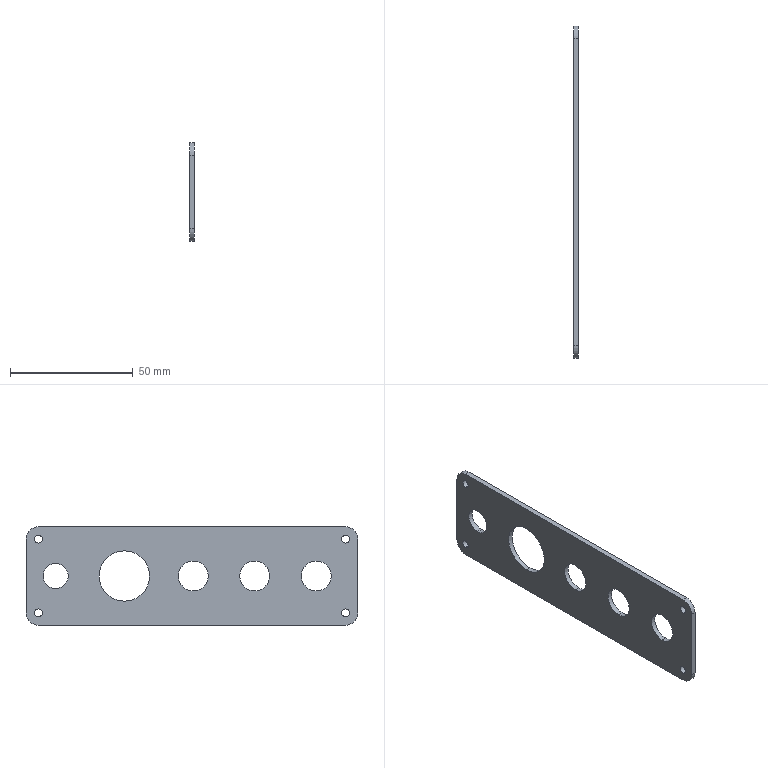Part | SolidWorks | features BaseBody 1 | 1 solid | 28 faces | box 2 x 135 x 40 mm | volume 9168 mm3 | cylinder 22 | plane 6 | commonest cylinder face diameters 3.2 x8 12.2 x6 10 x4 10.2 x2 20.5 x2
STEP:
#1=CARTESIAN_POINT('',(330.1,5.5,36.9));
#2=VERTEX_POINT('',#1);
#3=CARTESIAN_POINT('',(330.1,5.5,40.1));
#4=VERTEX_POINT('',#3);
#5=CARTESIAN_POINT('',(330.1,5.5,38.5));
#6=DIRECTION('',(-1.,0.,0.));
#7=DIRECTION('',(0.,0.,1.));
#8=AXIS2_PLACEMENT_3D('',#5,#6,#7);
#9=CIRCLE('',#8,1.6);
#10=EDGE_CURVE('',#2,#4,#9,.T.);
#11=ORIENTED_EDGE('',*,*,#10,.F.);
#12=CARTESIAN_POINT('',(328.1,5.5,36.9));
#13=VERTEX_POINT('',#12);
#14=CARTESIAN_POINT('',(330.1,5.5,36.9));
#15=DIRECTION('',(-1.,0.,0.));
#16=VECTOR('',#15,1000.);
#17=LINE('',#14,#16);
#18=EDGE_CURVE('',#2,#13,#17,.T.);
#19=ORIENTED_EDGE('',*,*,#18,.T.);
#20=CARTESIAN_POINT('',(328.1,5.5,40.1));
#21=VERTEX_POINT('',#20);
#22=CARTESIAN_POINT('',(328.1,5.5,38.5));
#23=DIRECTION('',(1.,0.,0.));
#24=DIRECTION('',(0.,0.,1.));
#25=AXIS2_PLACEMENT_3D('',#22,#23,#24);
#26=CIRCLE('',#25,1.6);
#27=EDGE_CURVE('',#21,#13,#26,.T.);
#28=ORIENTED_EDGE('',*,*,#27,.F.);
#29=CARTESIAN_POINT('',(330.1,5.5,40.1));
#30=DIRECTION('',(-1.,0.,0.));
#31=VECTOR('',#30,1000.);
#32=LINE('',#29,#31);
#33=EDGE_CURVE('',#4,#21,#32,.T.);
#34=ORIENTED_EDGE('',*,*,#33,.F.);
#35=EDGE_LOOP('',(#11,#19,#28,#34));
#36=FACE_OUTER_BOUND('',#35,.T.);
#37=CARTESIAN_POINT('',(330.1,5.5,38.5));
#38=DIRECTION('',(-1.,0.,0.));
#39=DIRECTION('',(0.,0.,1.));
#40=AXIS2_PLACEMENT_3D('',#37,#38,#39);
#41=CYLINDRICAL_SURFACE('',#40,1.6);
#42=ADVANCED_FACE('',(#36),#41,.F.);
#43=CARTESIAN_POINT('',(330.1,130.5,6.9));
#44=VERTEX_POINT('',#43);
#45=CARTESIAN_POINT('',(330.1,130.5,10.1));
#46=VERTEX_POINT('',#45);
#47=CARTESIAN_POINT('',(330.1,130.5,8.5));
#48=DIRECTION('',(-1.,0.,0.));
#49=DIRECTION('',(0.,0.,1.));
#50=AXIS2_PLACEMENT_3D('',#47,#48,#49);
#51=CIRCLE('',#50,1.6);
#52=EDGE_CURVE('',#44,#46,#51,.T.);
#53=ORIENTED_EDGE('',*,*,#52,.F.);
#54=CARTESIAN_POINT('',(328.1,130.5,6.9));
#55=VERTEX_POINT('',#54);
#56=CARTESIAN_POINT('',(330.1,130.5,6.9));
#57=DIRECTION('',(-1.,0.,0.));
#58=VECTOR('',#57,1000.);
#59=LINE('',#56,#58);
#60=EDGE_CURVE('',#44,#55,#59,.T.);
#61=ORIENTED_EDGE('',*,*,#60,.T.);
#62=CARTESIAN_POINT('',(328.1,130.5,10.1));
#63=VERTEX_POINT('',#62);
#64=CARTESIAN_POINT('',(328.1,130.5,8.5));
#65=DIRECTION('',(1.,0.,0.));
#66=DIRECTION('',(0.,0.,1.));
#67=AXIS2_PLACEMENT_3D('',#64,#65,#66);
#68=CIRCLE('',#67,1.6);
#69=EDGE_CURVE('',#63,#55,#68,.T.);
#70=ORIENTED_EDGE('',*,*,#69,.F.);
#71=CARTESIAN_POINT('',(330.1,130.5,10.1));
#72=DIRECTION('',(-1.,0.,0.));
#73=VECTOR('',#72,1000.);
#74=LINE('',#71,#73);
#75=EDGE_CURVE('',#46,#63,#74,.T.);
#76=ORIENTED_EDGE('',*,*,#75,.F.);
#77=EDGE_LOOP('',(#53,#61,#70,#76));
#78=FACE_OUTER_BOUND('',#77,.T.);
#79=CARTESIAN_POINT('',(330.1,130.5,8.5));
#80=DIRECTION('',(-1.,0.,0.));
#81=DIRECTION('',(0.,0.,1.));
#82=AXIS2_PLACEMENT_3D('',#79,#80,#81);
#83=CYLINDRICAL_SURFACE('',#82,1.6);
#84=ADVANCED_FACE('',(#78),#83,.F.);
#85=CARTESIAN_POINT('',(330.1,130.5,36.9));
#86=VERTEX_POINT('',#85);
#87=CARTESIAN_POINT('',(330.1,130.5,40.1));
#88=VERTEX_POINT('',#87);
#89=CARTESIAN_POINT('',(330.1,130.5,38.5));
#90=DIRECTION('',(-1.,0.,0.));
#91=DIRECTION('',(0.,0.,1.));
#92=AXIS2_PLACEMENT_3D('',#89,#90,#91);
#93=CIRCLE('',#92,1.6);
#94=EDGE_CURVE('',#86,#88,#93,.T.);
#95=ORIENTED_EDGE('',*,*,#94,.F.);
#96=CARTESIAN_POINT('',(328.1,130.5,36.9));
#97=VERTEX_POINT('',#96);
#98=CARTESIAN_POINT('',(330.1,130.5,36.9));
#99=DIRECTION('',(-1.,0.,0.));
#100=VECTOR('',#99,1000.);
#101=LINE('',#98,#100);
#102=EDGE_CURVE('',#86,#97,#101,.T.);
#103=ORIENTED_EDGE('',*,*,#102,.T.);
#104=CARTESIAN_POINT('',(328.1,130.5,40.1));
#105=VERTEX_POINT('',#104);
#106=CARTESIAN_POINT('',(328.1,130.5,38.5));
#107=DIRECTION('',(1.,0.,0.));
#108=DIRECTION('',(0.,0.,1.));
#109=AXIS2_PLACEMENT_3D('',#106,#107,#108);
#110=CIRCLE('',#109,1.6);
#111=EDGE_CURVE('',#105,#97,#110,.T.);
#112=ORIENTED_EDGE('',*,*,#111,.F.);
#113=CARTESIAN_POINT('',(330.1,130.5,40.1));
#114=DIRECTION('',(-1.,0.,0.));
#115=VECTOR('',#114,1000.);
#116=LINE('',#113,#115);
#117=EDGE_CURVE('',#88,#105,#116,.T.);
#118=ORIENTED_EDGE('',*,*,#117,.F.);
#119=EDGE_LOOP('',(#95,#103,#112,#118));
#120=FACE_OUTER_BOUND('',#119,.T.);
#121=CARTESIAN_POINT('',(330.1,130.5,38.5));
#122=DIRECTION('',(-1.,0.,0.));
#123=DIRECTION('',(0.,0.,1.));
#124=AXIS2_PLACEMENT_3D('',#121,#122,#123);
#125=CYLINDRICAL_SURFACE('',#124,1.6);
#126=ADVANCED_FACE('',(#120),#125,.F.);
#127=CARTESIAN_POINT('',(330.1,5.5,6.9));
#128=VERTEX_POINT('',#127);
#129=CARTESIAN_POINT('',(330.1,5.5,10.1));
#130=VERTEX_POINT('',#129);
#131=CARTESIAN_POINT('',(330.1,5.5,8.5));
#132=DIRECTION('',(-1.,0.,0.));
#133=DIRECTION('',(0.,0.,1.));
#134=AXIS2_PLACEMENT_3D('',#131,#132,#133);
#135=CIRCLE('',#134,1.6);
#136=EDGE_CURVE('',#128,#130,#135,.T.);
#137=ORIENTED_EDGE('',*,*,#136,.F.);
#138=CARTESIAN_POINT('',(328.1,5.5,6.9));
#139=VERTEX_POINT('',#138);
#140=CARTESIAN_POINT('',(330.1,5.5,6.9));
#141=DIRECTION('',(-1.,0.,0.));
#142=VECTOR('',#141,1000.);
#143=LINE('',#140,#142);
#144=EDGE_CURVE('',#128,#139,#143,.T.);
#145=ORIENTED_EDGE('',*,*,#144,.T.);
#146=CARTESIAN_POINT('',(328.1,5.5,10.1));
#147=VERTEX_POINT('',#146);
#148=CARTESIAN_POINT('',(328.1,5.5,8.5));
#149=DIRECTION('',(1.,0.,0.));
#150=DIRECTION('',(0.,0.,1.));
#151=AXIS2_PLACEMENT_3D('',#148,#149,#150);
#152=CIRCLE('',#151,1.6);
#153=EDGE_CURVE('',#147,#139,#152,.T.);
#154=ORIENTED_EDGE('',*,*,#153,.F.);
#155=CARTESIAN_POINT('',(330.1,5.5,10.1));
#156=DIRECTION('',(-1.,0.,0.));
#157=VECTOR('',#156,1000.);
#158=LINE('',#155,#157);
#159=EDGE_CURVE('',#130,#147,#158,.T.);
#160=ORIENTED_EDGE('',*,*,#159,.F.);
#161=EDGE_LOOP('',(#137,#145,#154,#160));
#162=FACE_OUTER_BOUND('',#161,.T.);
#163=CARTESIAN_POINT('',(330.1,5.5,8.5));
#164=DIRECTION('',(-1.,0.,0.));
#165=DIRECTION('',(0.,0.,1.));
#166=AXIS2_PLACEMENT_3D('',#163,#164,#165);
#167=CYLINDRICAL_SURFACE('',#166,1.6);
#168=ADVANCED_FACE('',(#162),#167,.F.);
#169=CARTESIAN_POINT('',(330.1,95.5,13.25));
#170=VERTEX_POINT('',#169);
#171=CARTESIAN_POINT('',(330.1,95.5,33.75));
#172=VERTEX_POINT('',#171);
#173=CARTESIAN_POINT('',(330.1,95.5,23.5));
#174=DIRECTION('',(-1.,0.,0.));
#175=DIRECTION('',(0.,0.,1.));
#176=AXIS2_PLACEMENT_3D('',#173,#174,#175);
#177=CIRCLE('',#176,10.25);
#178=EDGE_CURVE('',#170,#172,#177,.T.);
#179=ORIENTED_EDGE('',*,*,#178,.F.);
#180=CARTESIAN_POINT('',(328.1,95.5,13.25));
#181=VERTEX_POINT('',#180);
#182=CARTESIAN_POINT('',(342.1,95.5,13.25));
#183=DIRECTION('',(-1.,0.,0.));
#184=VECTOR('',#183,1000.);
#185=LINE('',#182,#184);
#186=EDGE_CURVE('',#170,#181,#185,.T.);
#187=ORIENTED_EDGE('',*,*,#186,.T.);
#188=CARTESIAN_POINT('',(328.1,95.5,33.75));
#189=VERTEX_POINT('',#188);
#190=CARTESIAN_POINT('',(328.1,95.5,23.5));
#191=DIRECTION('',(1.,0.,0.));
#192=DIRECTION('',(0.,0.,1.));
#193=AXIS2_PLACEMENT_3D('',#190,#191,#192);
#194=CIRCLE('',#193,10.25);
#195=EDGE_CURVE('',#189,#181,#194,.T.);
#196=ORIENTED_EDGE('',*,*,#195,.F.);
#197=CARTESIAN_POINT('',(342.1,95.5,33.75));
#198=DIRECTION('',(-1.,0.,0.));
#199=VECTOR('',#198,1000.);
#200=LINE('',#197,#199);
#201=EDGE_CURVE('',#172,#189,#200,.T.);
#202=ORIENTED_EDGE('',*,*,#201,.F.);
#203=EDGE_LOOP('',(#179,#187,#196,#202));
#204=FACE_OUTER_BOUND('',#203,.T.);
#205=CARTESIAN_POINT('',(342.1,95.5,23.5));
#206=DIRECTION('',(-1.,0.,0.));
#207=DIRECTION('',(0.,0.,1.));
#208=AXIS2_PLACEMENT_3D('',#205,#206,#207);
#209=CYLINDRICAL_SURFACE('',#208,10.25);
#210=ADVANCED_FACE('',(#204),#209,.F.);
#211=CARTESIAN_POINT('',(330.1,123.5,18.4));
#212=VERTEX_POINT('',#211);
#213=CARTESIAN_POINT('',(330.1,123.5,28.6));
#214=VERTEX_POINT('',#213);
#215=CARTESIAN_POINT('',(330.1,123.5,23.5));
#216=DIRECTION('',(-1.,0.,0.));
#217=DIRECTION('',(0.,0.,1.));
#218=AXIS2_PLACEMENT_3D('',#215,#216,#217);
#219=CIRCLE('',#218,5.1);
#220=EDGE_CURVE('',#212,#214,#219,.T.);
#221=ORIENTED_EDGE('',*,*,#220,.F.);
#222=CARTESIAN_POINT('',(328.1,123.5,18.4));
#223=VERTEX_POINT('',#222);
#224=CARTESIAN_POINT('',(330.1,123.5,18.4));
#225=DIRECTION('',(-1.,0.,0.));
#226=VECTOR('',#225,1000.);
#227=LINE('',#224,#226);
#228=EDGE_CURVE('',#212,#223,#227,.T.);
#229=ORIENTED_EDGE('',*,*,#228,.T.);
#230=CARTESIAN_POINT('',(328.1,123.5,28.6));
#231=VERTEX_POINT('',#230);
#232=CARTESIAN_POINT('',(328.1,123.5,23.5));
#233=DIRECTION('',(1.,0.,0.));
#234=DIRECTION('',(0.,0.,1.));
#235=AXIS2_PLACEMENT_3D('',#232,#233,#234);
#236=CIRCLE('',#235,5.1);
#237=EDGE_CURVE('',#231,#223,#236,.T.);
#238=ORIENTED_EDGE('',*,*,#237,.F.);
#239=CARTESIAN_POINT('',(330.1,123.5,28.6));
#240=DIRECTION('',(-1.,0.,0.));
#241=VECTOR('',#240,1000.);
#242=LINE('',#239,#241);
#243=EDGE_CURVE('',#214,#231,#242,.T.);
#244=ORIENTED_EDGE('',*,*,#243,.F.);
#245=EDGE_LOOP('',(#221,#229,#238,#244));
#246=FACE_OUTER_BOUND('',#245,.T.);
#247=CARTESIAN_POINT('',(330.1,123.5,23.5));
#248=DIRECTION('',(-1.,0.,0.));
#249=DIRECTION('',(0.,0.,1.));
#250=AXIS2_PLACEMENT_3D('',#247,#248,#249);
#251=CYLINDRICAL_SURFACE('',#250,5.1);
#252=ADVANCED_FACE('',(#246),#251,.F.);
#253=CARTESIAN_POINT('',(330.1,67.5,17.4));
#254=VERTEX_POINT('',#253);
#255=CARTESIAN_POINT('',(330.1,67.5,29.6));
#256=VERTEX_POINT('',#255);
#257=CARTESIAN_POINT('',(330.1,67.5,23.5));
#258=DIRECTION('',(-1.,0.,0.));
#259=DIRECTION('',(0.,0.,1.));
#260=AXIS2_PLACEMENT_3D('',#257,#258,#259);
#261=CIRCLE('',#260,6.1);
#262=EDGE_CURVE('',#254,#256,#261,.T.);
#263=ORIENTED_EDGE('',*,*,#262,.F.);
#264=CARTESIAN_POINT('',(328.1,67.5,17.4));
#265=VERTEX_POINT('',#264);
#266=CARTESIAN_POINT('',(342.1,67.5,17.4));
#267=DIRECTION('',(-1.,0.,0.));
#268=VECTOR('',#267,1000.);
#269=LINE('',#266,#268);
#270=EDGE_CURVE('',#254,#265,#269,.T.);
#271=ORIENTED_EDGE('',*,*,#270,.T.);
#272=CARTESIAN_POINT('',(328.1,67.5,29.6));
#273=VERTEX_POINT('',#272);
#274=CARTESIAN_POINT('',(328.1,67.5,23.5));
#275=DIRECTION('',(1.,0.,0.));
#276=DIRECTION('',(0.,0.,1.));
#277=AXIS2_PLACEMENT_3D('',#274,#275,#276);
#278=CIRCLE('',#277,6.1);
#279=EDGE_CURVE('',#273,#265,#278,.T.);
#280=ORIENTED_EDGE('',*,*,#279,.F.);
#281=CARTESIAN_POINT('',(342.1,67.5,29.6));
#282=DIRECTION('',(-1.,0.,0.));
#283=VECTOR('',#282,1000.);
#284=LINE('',#281,#283);
#285=EDGE_CURVE('',#256,#273,#284,.T.);
#286=ORIENTED_EDGE('',*,*,#285,.F.);
#287=EDGE_LOOP('',(#263,#271,#280,#286));
#288=FACE_OUTER_BOUND('',#287,.T.);
#289=CARTESIAN_POINT('',(342.1,67.5,23.5));
#290=DIRECTION('',(-1.,0.,0.));
#291=DIRECTION('',(0.,0.,1.));
#292=AXIS2_PLACEMENT_3D('',#289,#290,#291);
#293=CYLINDRICAL_SURFACE('',#292,6.1);
#294=ADVANCED_FACE('',(#288),#293,.F.);
#295=CARTESIAN_POINT('',(330.1,42.5,17.4));
#296=VERTEX_POINT('',#295);
#297=CARTESIAN_POINT('',(330.1,42.5,29.6));
#298=VERTEX_POINT('',#297);
#299=CARTESIAN_POINT('',(330.1,42.5,23.5));
#300=DIRECTION('',(-1.,0.,0.));
#301=DIRECTION('',(0.,0.,1.));
#302=AXIS2_PLACEMENT_3D('',#299,#300,#301);
#303=CIRCLE('',#302,6.1);
#304=EDGE_CURVE('',#296,#298,#303,.T.);
#305=ORIENTED_EDGE('',*,*,#304,.F.);
#306=CARTESIAN_POINT('',(328.1,42.5,17.4));
#307=VERTEX_POINT('',#306);
#308=CARTESIAN_POINT('',(342.1,42.5,17.4));
#309=DIRECTION('',(-1.,0.,0.));
#310=VECTOR('',#309,1000.);
#311=LINE('',#308,#310);
#312=EDGE_CURVE('',#296,#307,#311,.T.);
#313=ORIENTED_EDGE('',*,*,#312,.T.);
#314=CARTESIAN_POINT('',(328.1,42.5,29.6));
#315=VERTEX_POINT('',#314);
#316=CARTESIAN_POINT('',(328.1,42.5,23.5));
#317=DIRECTION('',(1.,0.,0.));
#318=DIRECTION('',(0.,0.,1.));
#319=AXIS2_PLACEMENT_3D('',#316,#317,#318);
#320=CIRCLE('',#319,6.1);
#321=EDGE_CURVE('',#315,#307,#320,.T.);
#322=ORIENTED_EDGE('',*,*,#321,.F.);
#323=CARTESIAN_POINT('',(342.1,42.5,29.6));
#324=DIRECTION('',(-1.,0.,0.));
#325=VECTOR('',#324,1000.);
#326=LINE('',#323,#325);
#327=EDGE_CURVE('',#298,#315,#326,.T.);
#328=ORIENTED_EDGE('',*,*,#327,.F.);
#329=EDGE_LOOP('',(#305,#313,#322,#328));
#330=FACE_OUTER_BOUND('',#329,.T.);
#331=CARTESIAN_POINT('',(342.1,42.5,23.5));
#332=DIRECTION('',(-1.,0.,0.));
#333=DIRECTION('',(0.,0.,1.));
#334=AXIS2_PLACEMENT_3D('',#331,#332,#333);
#335=CYLINDRICAL_SURFACE('',#334,6.1);
#336=ADVANCED_FACE('',(#330),#335,.F.);
#337=CARTESIAN_POINT('',(330.1,17.5,17.4));
#338=VERTEX_POINT('',#337);
#339=CARTESIAN_POINT('',(330.1,17.5,29.6));
#340=VERTEX_POINT('',#339);
#341=CARTESIAN_POINT('',(330.1,17.5,23.5));
#342=DIRECTION('',(-1.,0.,0.));
#343=DIRECTION('',(0.,0.,1.));
#344=AXIS2_PLACEMENT_3D('',#341,#342,#343);
#345=CIRCLE('',#344,6.1);
#346=EDGE_CURVE('',#338,#340,#345,.T.);
#347=ORIENTED_EDGE('',*,*,#346,.F.);
#348=CARTESIAN_POINT('',(328.1,17.5,17.4));
#349=VERTEX_POINT('',#348);
#350=CARTESIAN_POINT('',(342.1,17.5,17.4));
#351=DIRECTION('',(-1.,0.,0.));
#352=VECTOR('',#351,1000.);
#353=LINE('',#350,#352);
#354=EDGE_CURVE('',#338,#349,#353,.T.);
#355=ORIENTED_EDGE('',*,*,#354,.T.);
#356=CARTESIAN_POINT('',(328.1,17.5,29.6));
#357=VERTEX_POINT('',#356);
#358=CARTESIAN_POINT('',(328.1,17.5,23.5));
#359=DIRECTION('',(1.,0.,0.));
#360=DIRECTION('',(0.,0.,1.));
#361=AXIS2_PLACEMENT_3D('',#358,#359,#360);
#362=CIRCLE('',#361,6.1);
#363=EDGE_CURVE('',#357,#349,#362,.T.);
#364=ORIENTED_EDGE('',*,*,#363,.F.);
#365=CARTESIAN_POINT('',(342.1,17.5,29.6));
#366=DIRECTION('',(-1.,0.,0.));
#367=VECTOR('',#366,1000.);
#368=LINE('',#365,#367);
#369=EDGE_CURVE('',#340,#357,#368,.T.);
#370=ORIENTED_EDGE('',*,*,#369,.F.);
#371=EDGE_LOOP('',(#347,#355,#364,#370));
#372=FACE_OUTER_BOUND('',#371,.T.);
#373=CARTESIAN_POINT('',(342.1,17.5,23.5));
#374=DIRECTION('',(-1.,0.,0.));
#375=DIRECTION('',(0.,0.,1.));
#376=AXIS2_PLACEMENT_3D('',#373,#374,#375);
#377=CYLINDRICAL_SURFACE('',#376,6.1);
#378=ADVANCED_FACE('',(#372),#377,.F.);
#379=CARTESIAN_POINT('',(330.1,17.5,23.5));
#380=DIRECTION('',(-1.,0.,0.));
#381=DIRECTION('',(0.,0.,1.));
#382=AXIS2_PLACEMENT_3D('',#379,#380,#381);
#383=CIRCLE('',#382,6.1);
#384=EDGE_CURVE('',#340,#338,#383,.T.);
#385=ORIENTED_EDGE('',*,*,#384,.T.);
#386=ORIENTED_EDGE('',*,*,#346,.T.);
#387=EDGE_LOOP('',(#385,#386));
#388=FACE_BOUND('',#387,.T.);
#389=CARTESIAN_POINT('',(330.1,95.5,23.5));
#390=DIRECTION('',(-1.,0.,0.));
#391=DIRECTION('',(0.,0.,1.));
#392=AXIS2_PLACEMENT_3D('',#389,#390,#391);
#393=CIRCLE('',#392,10.25);
#394=EDGE_CURVE('',#172,#170,#393,.T.);
#395=ORIENTED_EDGE('',*,*,#394,.T.);
#396=ORIENTED_EDGE('',*,*,#178,.T.);
#397=EDGE_LOOP('',(#395,#396));
#398=FACE_BOUND('',#397,.T.);
#399=CARTESIAN_POINT('',(330.1,123.5,23.5));
#400=DIRECTION('',(-1.,0.,0.));
#401=DIRECTION('',(0.,0.,1.));
#402=AXIS2_PLACEMENT_3D('',#399,#400,#401);
#403=CIRCLE('',#402,5.1);
#404=EDGE_CURVE('',#214,#212,#403,.T.);
#405=ORIENTED_EDGE('',*,*,#404,.T.);
#406=ORIENTED_EDGE('',*,*,#220,.T.);
#407=EDGE_LOOP('',(#405,#406));
#408=FACE_BOUND('',#407,.T.);
#409=CARTESIAN_POINT('',(330.1,67.5,23.5));
#410=DIRECTION('',(-1.,0.,0.));
#411=DIRECTION('',(0.,0.,1.));
#412=AXIS2_PLACEMENT_3D('',#409,#410,#411);
#413=CIRCLE('',#412,6.1);
#414=EDGE_CURVE('',#256,#254,#413,.T.);
#415=ORIENTED_EDGE('',*,*,#414,.T.);
#416=ORIENTED_EDGE('',*,*,#262,.T.);
#417=EDGE_LOOP('',(#415,#416));
#418=FACE_BOUND('',#417,.T.);
#419=CARTESIAN_POINT('',(330.1,42.5,23.5));
#420=DIRECTION('',(-1.,0.,0.));
#421=DIRECTION('',(0.,0.,1.));
#422=AXIS2_PLACEMENT_3D('',#419,#420,#421);
#423=CIRCLE('',#422,6.1);
#424=EDGE_CURVE('',#298,#296,#423,.T.);
#425=ORIENTED_EDGE('',*,*,#424,.T.);
#426=ORIENTED_EDGE('',*,*,#304,.T.);
#427=EDGE_LOOP('',(#425,#426));
#428=FACE_BOUND('',#427,.T.);
#429=CARTESIAN_POINT('',(330.1,5.5,8.5));
#430=DIRECTION('',(-1.,0.,0.));
#431=DIRECTION('',(0.,0.,1.));
#432=AXIS2_PLACEMENT_3D('',#429,#430,#431);
#433=CIRCLE('',#432,1.6);
#434=EDGE_CURVE('',#130,#128,#433,.T.);
#435=ORIENTED_EDGE('',*,*,#434,.T.);
#436=ORIENTED_EDGE('',*,*,#136,.T.);
#437=EDGE_LOOP('',(#435,#436));
#438=FACE_BOUND('',#437,.T.);
#439=CARTESIAN_POINT('',(330.1,130.5,38.5));
#440=DIRECTION('',(-1.,0.,0.));
#441=DIRECTION('',(0.,0.,1.));
#442=AXIS2_PLACEMENT_3D('',#439,#440,#441);
#443=CIRCLE('',#442,1.6);
#444=EDGE_CURVE('',#88,#86,#443,.T.);
#445=ORIENTED_EDGE('',*,*,#444,.T.);
#446=ORIENTED_EDGE('',*,*,#94,.T.);
#447=EDGE_LOOP('',(#445,#446));
#448=FACE_BOUND('',#447,.T.);
#449=CARTESIAN_POINT('',(330.1,130.5,8.5));
#450=DIRECTION('',(-1.,0.,0.));
#451=DIRECTION('',(0.,0.,1.));
#452=AXIS2_PLACEMENT_3D('',#449,#450,#451);
#453=CIRCLE('',#452,1.6);
#454=EDGE_CURVE('',#46,#44,#453,.T.);
#455=ORIENTED_EDGE('',*,*,#454,.T.);
#456=ORIENTED_EDGE('',*,*,#52,.T.);
#457=EDGE_LOOP('',(#455,#456));
#458=FACE_BOUND('',#457,.T.);
#459=CARTESIAN_POINT('',(330.1,5.5,38.5));
#460=DIRECTION('',(-1.,0.,0.));
#461=DIRECTION('',(0.,0.,1.));
#462=AXIS2_PLACEMENT_3D('',#459,#460,#461);
#463=CIRCLE('',#462,1.6);
#464=EDGE_CURVE('',#4,#2,#463,.T.);
#465=ORIENTED_EDGE('',*,*,#464,.T.);
#466=ORIENTED_EDGE('',*,*,#10,.T.);
#467=EDGE_LOOP('',(#465,#466));
#468=FACE_BOUND('',#467,.T.);
#469=CARTESIAN_POINT('',(330.1,135.5,8.5));
#470=VERTEX_POINT('',#469);
#471=CARTESIAN_POINT('',(330.1,130.5,3.5));
#472=VERTEX_POINT('',#471);
#473=CARTESIAN_POINT('',(330.1,130.5,8.5));
#474=DIRECTION('',(-1.,0.,0.));
#475=DIRECTION('',(0.,0.,1.));
#476=AXIS2_PLACEMENT_3D('',#473,#474,#475);
#477=CIRCLE('',#476,5.);
#478=EDGE_CURVE('',#470,#472,#477,.T.);
#479=ORIENTED_EDGE('',*,*,#478,.F.);
#480=CARTESIAN_POINT('',(330.1,135.5,38.5));
#481=VERTEX_POINT('',#480);
#482=CARTESIAN_POINT('',(330.1,135.5,38.5));
#483=DIRECTION('',(0.,0.,1.));
#484=VECTOR('',#483,1000.);
#485=LINE('',#482,#484);
#486=EDGE_CURVE('',#470,#481,#485,.T.);
#487=ORIENTED_EDGE('',*,*,#486,.T.);
#488=CARTESIAN_POINT('',(330.1,130.5,43.5));
#489=VERTEX_POINT('',#488);
#490=CARTESIAN_POINT('',(330.1,130.5,38.5));
#491=DIRECTION('',(-1.,0.,0.));
#492=DIRECTION('',(0.,0.,1.));
#493=AXIS2_PLACEMENT_3D('',#490,#491,#492);
#494=CIRCLE('',#493,5.);
#495=EDGE_CURVE('',#489,#481,#494,.T.);
#496=ORIENTED_EDGE('',*,*,#495,.F.);
#497=CARTESIAN_POINT('',(330.1,5.5,43.5));
#498=VERTEX_POINT('',#497);
#499=CARTESIAN_POINT('',(330.1,3.5,43.5));
#500=DIRECTION('',(0.,-1.,0.));
#501=VECTOR('',#500,1000.);
#502=LINE('',#499,#501);
#503=EDGE_CURVE('',#489,#498,#502,.T.);
#504=ORIENTED_EDGE('',*,*,#503,.T.);
#505=CARTESIAN_POINT('',(330.1,0.5,38.5));
#506=VERTEX_POINT('',#505);
#507=CARTESIAN_POINT('',(330.1,5.5,38.5));
#508=DIRECTION('',(-1.,0.,0.));
#509=DIRECTION('',(0.,0.,1.));
#510=AXIS2_PLACEMENT_3D('',#507,#508,#509);
#511=CIRCLE('',#510,5.);
#512=EDGE_CURVE('',#506,#498,#511,.T.);
#513=ORIENTED_EDGE('',*,*,#512,.F.);
#514=CARTESIAN_POINT('',(330.1,0.5,8.5));
#515=VERTEX_POINT('',#514);
#516=CARTESIAN_POINT('',(330.1,0.5,38.5));
#517=DIRECTION('',(0.,0.,-1.));
#518=VECTOR('',#517,1000.);
#519=LINE('',#516,#518);
#520=EDGE_CURVE('',#506,#515,#519,.T.);
#521=ORIENTED_EDGE('',*,*,#520,.T.);
#522=CARTESIAN_POINT('',(330.1,5.5,3.5));
#523=VERTEX_POINT('',#522);
#524=CARTESIAN_POINT('',(330.1,5.5,8.5));
#525=DIRECTION('',(-1.,0.,0.));
#526=DIRECTION('',(0.,0.,1.));
#527=AXIS2_PLACEMENT_3D('',#524,#525,#526);
#528=CIRCLE('',#527,5.);
#529=EDGE_CURVE('',#523,#515,#528,.T.);
#530=ORIENTED_EDGE('',*,*,#529,.F.);
#531=CARTESIAN_POINT('',(330.1,3.5,3.5));
#532=DIRECTION('',(0.,1.,0.));
#533=VECTOR('',#532,1000.);
#534=LINE('',#531,#533);
#535=EDGE_CURVE('',#523,#472,#534,.T.);
#536=ORIENTED_EDGE('',*,*,#535,.T.);
#537=EDGE_LOOP('',(#479,#487,#496,#504,#513,#521,#530,#536));
#538=FACE_OUTER_BOUND('',#537,.T.);
#539=CARTESIAN_POINT('',(330.1,85.5,38.5));
#540=DIRECTION('',(-1.,0.,0.));
#541=DIRECTION('',(0.,0.,1.));
#542=AXIS2_PLACEMENT_3D('',#539,#540,#541);
#543=PLANE('',#542);
#544=ADVANCED_FACE('',(#388,#398,#408,#418,#428,#438,#448,#458,#468,#538),#543,.F.);
#545=CARTESIAN_POINT('',(328.1,0.5,38.5));
#546=VERTEX_POINT('',#545);
#547=CARTESIAN_POINT('',(330.1,0.5,38.5));
#548=DIRECTION('',(1.,0.,0.));
#549=VECTOR('',#548,1000.);
#550=LINE('',#547,#549);
#551=EDGE_CURVE('',#546,#506,#550,.T.);
#552=ORIENTED_EDGE('',*,*,#551,.F.);
#553=CARTESIAN_POINT('',(328.1,0.5,8.5));
#554=VERTEX_POINT('',#553);
#555=CARTESIAN_POINT('',(328.1,0.5,38.5));
#556=DIRECTION('',(0.,0.,1.));
#557=VECTOR('',#556,1000.);
#558=LINE('',#555,#557);
#559=EDGE_CURVE('',#554,#546,#558,.T.);
#560=ORIENTED_EDGE('',*,*,#559,.F.);
#561=CARTESIAN_POINT('',(330.1,0.5,8.5));
#562=DIRECTION('',(-1.,0.,0.));
#563=VECTOR('',#562,1000.);
#564=LINE('',#561,#563);
#565=EDGE_CURVE('',#515,#554,#564,.T.);
#566=ORIENTED_EDGE('',*,*,#565,.F.);
#567=ORIENTED_EDGE('',*,*,#520,.F.);
#568=EDGE_LOOP('',(#552,#560,#566,#567));
#569=FACE_OUTER_BOUND('',#568,.T.);
#570=CARTESIAN_POINT('',(330.1,0.5,38.5));
#571=DIRECTION('',(0.,1.,0.));
#572=DIRECTION('',(1.,0.,0.));
#573=AXIS2_PLACEMENT_3D('',#570,#571,#572);
#574=PLANE('',#573);
#575=ADVANCED_FACE('',(#569),#574,.F.);
#576=ORIENTED_EDGE('',*,*,#551,.T.);
#577=ORIENTED_EDGE('',*,*,#512,.T.);
#578=CARTESIAN_POINT('',(328.1,5.5,43.5));
#579=VERTEX_POINT('',#578);
#580=CARTESIAN_POINT('',(330.1,5.5,43.5));
#581=DIRECTION('',(-1.,0.,0.));
#582=VECTOR('',#581,1000.);
#583=LINE('',#580,#582);
#584=EDGE_CURVE('',#498,#579,#583,.T.);
#585=ORIENTED_EDGE('',*,*,#584,.T.);
#586=CARTESIAN_POINT('',(328.1,5.5,38.5));
#587=DIRECTION('',(-1.,0.,0.));
#588=DIRECTION('',(0.,0.,1.));
#589=AXIS2_PLACEMENT_3D('',#586,#587,#588);
#590=CIRCLE('',#589,5.);
#591=EDGE_CURVE('',#546,#579,#590,.T.);
#592=ORIENTED_EDGE('',*,*,#591,.F.);
#593=EDGE_LOOP('',(#576,#577,#585,#592));
#594=FACE_OUTER_BOUND('',#593,.T.);
#595=CARTESIAN_POINT('',(330.1,5.5,38.5));
#596=DIRECTION('',(-1.,0.,0.));
#597=DIRECTION('',(0.,0.,1.));
#598=AXIS2_PLACEMENT_3D('',#595,#596,#597);
#599=CYLINDRICAL_SURFACE('',#598,5.);
#600=ADVANCED_FACE('',(#594),#599,.T.);
#601=CARTESIAN_POINT('',(328.1,130.5,43.5));
#602=VERTEX_POINT('',#601);
#603=CARTESIAN_POINT('',(328.1,85.5,43.5));
#604=DIRECTION('',(0.,1.,0.));
#605=VECTOR('',#604,1000.);
#606=LINE('',#603,#605);
#607=EDGE_CURVE('',#579,#602,#606,.T.);
#608=ORIENTED_EDGE('',*,*,#607,.F.);
#609=ORIENTED_EDGE('',*,*,#584,.F.);
#610=ORIENTED_EDGE('',*,*,#503,.F.);
#611=CARTESIAN_POINT('',(330.1,130.5,43.5));
#612=DIRECTION('',(1.,0.,0.));
#613=VECTOR('',#612,1000.);
#614=LINE('',#611,#613);
#615=EDGE_CURVE('',#602,#489,#614,.T.);
#616=ORIENTED_EDGE('',*,*,#615,.F.);
#617=EDGE_LOOP('',(#608,#609,#610,#616));
#618=FACE_OUTER_BOUND('',#617,.T.);
#619=CARTESIAN_POINT('',(330.1,3.5,43.5));
#620=DIRECTION('',(0.,0.,-1.));
#621=DIRECTION('',(0.,-1.,0.));
#622=AXIS2_PLACEMENT_3D('',#619,#620,#621);
#623=PLANE('',#622);
#624=ADVANCED_FACE('',(#618),#623,.F.);
#625=ORIENTED_EDGE('',*,*,#615,.T.);
#626=ORIENTED_EDGE('',*,*,#495,.T.);
#627=CARTESIAN_POINT('',(328.1,135.5,38.5));
#628=VERTEX_POINT('',#627);
#629=CARTESIAN_POINT('',(330.1,135.5,38.5));
#630=DIRECTION('',(-1.,0.,0.));
#631=VECTOR('',#630,1000.);
#632=LINE('',#629,#631);
#633=EDGE_CURVE('',#481,#628,#632,.T.);
#634=ORIENTED_EDGE('',*,*,#633,.T.);
#635=CARTESIAN_POINT('',(328.1,130.5,38.5));
#636=DIRECTION('',(-1.,0.,0.));
#637=DIRECTION('',(0.,0.,1.));
#638=AXIS2_PLACEMENT_3D('',#635,#636,#637);
#639=CIRCLE('',#638,5.);
#640=EDGE_CURVE('',#602,#628,#639,.T.);
#641=ORIENTED_EDGE('',*,*,#640,.F.);
#642=EDGE_LOOP('',(#625,#626,#634,#641));
#643=FACE_OUTER_BOUND('',#642,.T.);
#644=CARTESIAN_POINT('',(330.1,130.5,38.5));
#645=DIRECTION('',(-1.,0.,0.));
#646=DIRECTION('',(0.,0.,1.));
#647=AXIS2_PLACEMENT_3D('',#644,#645,#646);
#648=CYLINDRICAL_SURFACE('',#647,5.);
#649=ADVANCED_FACE('',(#643),#648,.T.);
#650=CARTESIAN_POINT('',(328.1,135.5,8.5));
#651=VERTEX_POINT('',#650);
#652=CARTESIAN_POINT('',(330.1,135.5,8.5));
#653=DIRECTION('',(1.,0.,0.));
#654=VECTOR('',#653,1000.);
#655=LINE('',#652,#654);
#656=EDGE_CURVE('',#651,#470,#655,.T.);
#657=ORIENTED_EDGE('',*,*,#656,.F.);
#658=CARTESIAN_POINT('',(328.1,135.5,38.5));
#659=DIRECTION('',(0.,0.,-1.));
#660=VECTOR('',#659,1000.);
#661=LINE('',#658,#660);
#662=EDGE_CURVE('',#628,#651,#661,.T.);
#663=ORIENTED_EDGE('',*,*,#662,.F.);
#664=ORIENTED_EDGE('',*,*,#633,.F.);
#665=ORIENTED_EDGE('',*,*,#486,.F.);
#666=EDGE_LOOP('',(#657,#663,#664,#665));
#667=FACE_OUTER_BOUND('',#666,.T.);
#668=CARTESIAN_POINT('',(330.1,135.5,38.5));
#669=DIRECTION('',(0.,-1.,0.));
#670=DIRECTION('',(0.,0.,-1.));
#671=AXIS2_PLACEMENT_3D('',#668,#669,#670);
#672=PLANE('',#671);
#673=ADVANCED_FACE('',(#667),#672,.F.);
#674=ORIENTED_EDGE('',*,*,#656,.T.);
#675=ORIENTED_EDGE('',*,*,#478,.T.);
#676=CARTESIAN_POINT('',(328.1,130.5,3.5));
#677=VERTEX_POINT('',#676);
#678=CARTESIAN_POINT('',(330.1,130.5,3.5));
#679=DIRECTION('',(-1.,0.,0.));
#680=VECTOR('',#679,1000.);
#681=LINE('',#678,#680);
#682=EDGE_CURVE('',#472,#677,#681,.T.);
#683=ORIENTED_EDGE('',*,*,#682,.T.);
#684=CARTESIAN_POINT('',(328.1,130.5,8.5));
#685=DIRECTION('',(-1.,0.,0.));
#686=DIRECTION('',(0.,0.,1.));
#687=AXIS2_PLACEMENT_3D('',#684,#685,#686);
#688=CIRCLE('',#687,5.);
#689=EDGE_CURVE('',#651,#677,#688,.T.);
#690=ORIENTED_EDGE('',*,*,#689,.F.);
#691=EDGE_LOOP('',(#674,#675,#683,#690));
#692=FACE_OUTER_BOUND('',#691,.T.);
#693=CARTESIAN_POINT('',(330.1,130.5,8.5));
#694=DIRECTION('',(-1.,0.,0.));
#695=DIRECTION('',(0.,0.,1.));
#696=AXIS2_PLACEMENT_3D('',#693,#694,#695);
#697=CYLINDRICAL_SURFACE('',#696,5.);
#698=ADVANCED_FACE('',(#692),#697,.T.);
#699=ORIENTED_EDGE('',*,*,#682,.F.);
#700=ORIENTED_EDGE('',*,*,#535,.F.);
#701=CARTESIAN_POINT('',(328.1,5.5,3.5));
#702=VERTEX_POINT('',#701);
#703=CARTESIAN_POINT('',(330.1,5.5,3.5));
#704=DIRECTION('',(1.,0.,0.));
#705=VECTOR('',#704,1000.);
#706=LINE('',#703,#705);
#707=EDGE_CURVE('',#702,#523,#706,.T.);
#708=ORIENTED_EDGE('',*,*,#707,.F.);
#709=CARTESIAN_POINT('',(328.1,85.5,3.5));
#710=DIRECTION('',(0.,-1.,0.));
#711=VECTOR('',#710,1000.);
#712=LINE('',#709,#711);
#713=EDGE_CURVE('',#677,#702,#712,.T.);
#714=ORIENTED_EDGE('',*,*,#713,.F.);
#715=EDGE_LOOP('',(#699,#700,#708,#714));
#716=FACE_OUTER_BOUND('',#715,.T.);
#717=CARTESIAN_POINT('',(330.1,3.5,3.5));
#718=DIRECTION('',(0.,0.,1.));
#719=DIRECTION('',(1.,0.,0.));
#720=AXIS2_PLACEMENT_3D('',#717,#718,#719);
#721=PLANE('',#720);
#722=ADVANCED_FACE('',(#716),#721,.F.);
#723=ORIENTED_EDGE('',*,*,#707,.T.);
#724=ORIENTED_EDGE('',*,*,#529,.T.);
#725=ORIENTED_EDGE('',*,*,#565,.T.);
#726=CARTESIAN_POINT('',(328.1,5.5,8.5));
#727=DIRECTION('',(-1.,0.,0.));
#728=DIRECTION('',(0.,0.,1.));
#729=AXIS2_PLACEMENT_3D('',#726,#727,#728);
#730=CIRCLE('',#729,5.);
#731=EDGE_CURVE('',#702,#554,#730,.T.);
#732=ORIENTED_EDGE('',*,*,#731,.F.);
#733=EDGE_LOOP('',(#723,#724,#725,#732));
#734=FACE_OUTER_BOUND('',#733,.T.);
#735=CARTESIAN_POINT('',(330.1,5.5,8.5));
#736=DIRECTION('',(-1.,0.,0.));
#737=DIRECTION('',(0.,0.,1.));
#738=AXIS2_PLACEMENT_3D('',#735,#736,#737);
#739=CYLINDRICAL_SURFACE('',#738,5.);
#740=ADVANCED_FACE('',(#734),#739,.T.);
#741=ORIENTED_EDGE('',*,*,#363,.T.);
#742=CARTESIAN_POINT('',(328.1,17.5,23.5));
#743=DIRECTION('',(1.,0.,0.));
#744=DIRECTION('',(0.,0.,1.));
#745=AXIS2_PLACEMENT_3D('',#742,#743,#744);
#746=CIRCLE('',#745,6.1);
#747=EDGE_CURVE('',#349,#357,#746,.T.);
#748=ORIENTED_EDGE('',*,*,#747,.T.);
#749=EDGE_LOOP('',(#741,#748));
#750=FACE_BOUND('',#749,.T.);
#751=ORIENTED_EDGE('',*,*,#321,.T.);
#752=CARTESIAN_POINT('',(328.1,42.5,23.5));
#753=DIRECTION('',(1.,0.,0.));
#754=DIRECTION('',(0.,0.,1.));
#755=AXIS2_PLACEMENT_3D('',#752,#753,#754);
#756=CIRCLE('',#755,6.1);
#757=EDGE_CURVE('',#307,#315,#756,.T.);
#758=ORIENTED_EDGE('',*,*,#757,.T.);
#759=EDGE_LOOP('',(#751,#758));
#760=FACE_BOUND('',#759,.T.);
#761=ORIENTED_EDGE('',*,*,#279,.T.);
#762=CARTESIAN_POINT('',(328.1,67.5,23.5));
#763=DIRECTION('',(1.,0.,0.));
#764=DIRECTION('',(0.,0.,1.));
#765=AXIS2_PLACEMENT_3D('',#762,#763,#764);
#766=CIRCLE('',#765,6.1);
#767=EDGE_CURVE('',#265,#273,#766,.T.);
#768=ORIENTED_EDGE('',*,*,#767,.T.);
#769=EDGE_LOOP('',(#761,#768));
#770=FACE_BOUND('',#769,.T.);
#771=ORIENTED_EDGE('',*,*,#237,.T.);
#772=CARTESIAN_POINT('',(328.1,123.5,23.5));
#773=DIRECTION('',(1.,0.,0.));
#774=DIRECTION('',(0.,0.,1.));
#775=AXIS2_PLACEMENT_3D('',#772,#773,#774);
#776=CIRCLE('',#775,5.1);
#777=EDGE_CURVE('',#223,#231,#776,.T.);
#778=ORIENTED_EDGE('',*,*,#777,.T.);
#779=EDGE_LOOP('',(#771,#778));
#780=FACE_BOUND('',#779,.T.);
#781=ORIENTED_EDGE('',*,*,#195,.T.);
#782=CARTESIAN_POINT('',(328.1,95.5,23.5));
#783=DIRECTION('',(1.,0.,0.));
#784=DIRECTION('',(0.,0.,1.));
#785=AXIS2_PLACEMENT_3D('',#782,#783,#784);
#786=CIRCLE('',#785,10.25);
#787=EDGE_CURVE('',#181,#189,#786,.T.);
#788=ORIENTED_EDGE('',*,*,#787,.T.);
#789=EDGE_LOOP('',(#781,#788));
#790=FACE_BOUND('',#789,.T.);
#791=ORIENTED_EDGE('',*,*,#153,.T.);
#792=CARTESIAN_POINT('',(328.1,5.5,8.5));
#793=DIRECTION('',(1.,0.,0.));
#794=DIRECTION('',(0.,0.,1.));
#795=AXIS2_PLACEMENT_3D('',#792,#793,#794);
#796=CIRCLE('',#795,1.6);
#797=EDGE_CURVE('',#139,#147,#796,.T.);
#798=ORIENTED_EDGE('',*,*,#797,.T.);
#799=EDGE_LOOP('',(#791,#798));
#800=FACE_BOUND('',#799,.T.);
#801=ORIENTED_EDGE('',*,*,#111,.T.);
#802=CARTESIAN_POINT('',(328.1,130.5,38.5));
#803=DIRECTION('',(1.,0.,0.));
#804=DIRECTION('',(0.,0.,1.));
#805=AXIS2_PLACEMENT_3D('',#802,#803,#804);
#806=CIRCLE('',#805,1.6);
#807=EDGE_CURVE('',#97,#105,#806,.T.);
#808=ORIENTED_EDGE('',*,*,#807,.T.);
#809=EDGE_LOOP('',(#801,#808));
#810=FACE_BOUND('',#809,.T.);
#811=ORIENTED_EDGE('',*,*,#69,.T.);
#812=CARTESIAN_POINT('',(328.1,130.5,8.5));
#813=DIRECTION('',(1.,0.,0.));
#814=DIRECTION('',(0.,0.,1.));
#815=AXIS2_PLACEMENT_3D('',#812,#813,#814);
#816=CIRCLE('',#815,1.6);
#817=EDGE_CURVE('',#55,#63,#816,.T.);
#818=ORIENTED_EDGE('',*,*,#817,.T.);
#819=EDGE_LOOP('',(#811,#818));
#820=FACE_BOUND('',#819,.T.);
#821=ORIENTED_EDGE('',*,*,#27,.T.);
#822=CARTESIAN_POINT('',(328.1,5.5,38.5));
#823=DIRECTION('',(1.,0.,0.));
#824=DIRECTION('',(0.,0.,1.));
#825=AXIS2_PLACEMENT_3D('',#822,#823,#824);
#826=CIRCLE('',#825,1.6);
#827=EDGE_CURVE('',#13,#21,#826,.T.);
#828=ORIENTED_EDGE('',*,*,#827,.T.);
#829=EDGE_LOOP('',(#821,#828));
#830=FACE_BOUND('',#829,.T.);
#831=ORIENTED_EDGE('',*,*,#713,.T.);
#832=ORIENTED_EDGE('',*,*,#731,.T.);
#833=ORIENTED_EDGE('',*,*,#559,.T.);
#834=ORIENTED_EDGE('',*,*,#591,.T.);
#835=ORIENTED_EDGE('',*,*,#607,.T.);
#836=ORIENTED_EDGE('',*,*,#640,.T.);
#837=ORIENTED_EDGE('',*,*,#662,.T.);
#838=ORIENTED_EDGE('',*,*,#689,.T.);
#839=EDGE_LOOP('',(#831,#832,#833,#834,#835,#836,#837,#838));
#840=FACE_OUTER_BOUND('',#839,.T.);
#841=CARTESIAN_POINT('',(328.1,85.5,38.5));
#842=DIRECTION('',(-1.,0.,0.));
#843=DIRECTION('',(0.,0.,1.));
#844=AXIS2_PLACEMENT_3D('',#841,#842,#843);
#845=PLANE('',#844);
#846=ADVANCED_FACE('',(#750,#760,#770,#780,#790,#800,#810,#820,#830,#840),#845,.T.);
#847=ORIENTED_EDGE('',*,*,#354,.F.);
#848=ORIENTED_EDGE('',*,*,#384,.F.);
#849=ORIENTED_EDGE('',*,*,#369,.T.);
#850=ORIENTED_EDGE('',*,*,#747,.F.);
#851=EDGE_LOOP('',(#847,#848,#849,#850));
#852=FACE_OUTER_BOUND('',#851,.T.);
#853=CARTESIAN_POINT('',(342.1,17.5,23.5));
#854=DIRECTION('',(-1.,0.,0.));
#855=DIRECTION('',(0.,0.,1.));
#856=AXIS2_PLACEMENT_3D('',#853,#854,#855);
#857=CYLINDRICAL_SURFACE('',#856,6.1);
#858=ADVANCED_FACE('',(#852),#857,.F.);
#859=ORIENTED_EDGE('',*,*,#312,.F.);
#860=ORIENTED_EDGE('',*,*,#424,.F.);
#861=ORIENTED_EDGE('',*,*,#327,.T.);
#862=ORIENTED_EDGE('',*,*,#757,.F.);
#863=EDGE_LOOP('',(#859,#860,#861,#862));
#864=FACE_OUTER_BOUND('',#863,.T.);
#865=CARTESIAN_POINT('',(342.1,42.5,23.5));
#866=DIRECTION('',(-1.,0.,0.));
#867=DIRECTION('',(0.,0.,1.));
#868=AXIS2_PLACEMENT_3D('',#865,#866,#867);
#869=CYLINDRICAL_SURFACE('',#868,6.1);
#870=ADVANCED_FACE('',(#864),#869,.F.);
#871=ORIENTED_EDGE('',*,*,#270,.F.);
#872=ORIENTED_EDGE('',*,*,#414,.F.);
#873=ORIENTED_EDGE('',*,*,#285,.T.);
#874=ORIENTED_EDGE('',*,*,#767,.F.);
#875=EDGE_LOOP('',(#871,#872,#873,#874));
#876=FACE_OUTER_BOUND('',#875,.T.);
#877=CARTESIAN_POINT('',(342.1,67.5,23.5));
#878=DIRECTION('',(-1.,0.,0.));
#879=DIRECTION('',(0.,0.,1.));
#880=AXIS2_PLACEMENT_3D('',#877,#878,#879);
#881=CYLINDRICAL_SURFACE('',#880,6.1);
#882=ADVANCED_FACE('',(#876),#881,.F.);
#883=ORIENTED_EDGE('',*,*,#228,.F.);
#884=ORIENTED_EDGE('',*,*,#404,.F.);
#885=ORIENTED_EDGE('',*,*,#243,.T.);
#886=ORIENTED_EDGE('',*,*,#777,.F.);
#887=EDGE_LOOP('',(#883,#884,#885,#886));
#888=FACE_OUTER_BOUND('',#887,.T.);
#889=CARTESIAN_POINT('',(330.1,123.5,23.5));
#890=DIRECTION('',(-1.,0.,0.));
#891=DIRECTION('',(0.,0.,1.));
#892=AXIS2_PLACEMENT_3D('',#889,#890,#891);
#893=CYLINDRICAL_SURFACE('',#892,5.1);
#894=ADVANCED_FACE('',(#888),#893,.F.);
#895=ORIENTED_EDGE('',*,*,#186,.F.);
#896=ORIENTED_EDGE('',*,*,#394,.F.);
#897=ORIENTED_EDGE('',*,*,#201,.T.);
#898=ORIENTED_EDGE('',*,*,#787,.F.);
#899=EDGE_LOOP('',(#895,#896,#897,#898));
#900=FACE_OUTER_BOUND('',#899,.T.);
#901=CARTESIAN_POINT('',(342.1,95.5,23.5));
#902=DIRECTION('',(-1.,0.,0.));
#903=DIRECTION('',(0.,0.,1.));
#904=AXIS2_PLACEMENT_3D('',#901,#902,#903);
#905=CYLINDRICAL_SURFACE('',#904,10.25);
#906=ADVANCED_FACE('',(#900),#905,.F.);
#907=ORIENTED_EDGE('',*,*,#144,.F.);
#908=ORIENTED_EDGE('',*,*,#434,.F.);
#909=ORIENTED_EDGE('',*,*,#159,.T.);
#910=ORIENTED_EDGE('',*,*,#797,.F.);
#911=EDGE_LOOP('',(#907,#908,#909,#910));
#912=FACE_OUTER_BOUND('',#911,.T.);
#913=CARTESIAN_POINT('',(330.1,5.5,8.5));
#914=DIRECTION('',(-1.,0.,0.));
#915=DIRECTION('',(0.,0.,1.));
#916=AXIS2_PLACEMENT_3D('',#913,#914,#915);
#917=CYLINDRICAL_SURFACE('',#916,1.6);
#918=ADVANCED_FACE('',(#912),#917,.F.);
#919=ORIENTED_EDGE('',*,*,#102,.F.);
#920=ORIENTED_EDGE('',*,*,#444,.F.);
#921=ORIENTED_EDGE('',*,*,#117,.T.);
#922=ORIENTED_EDGE('',*,*,#807,.F.);
#923=EDGE_LOOP('',(#919,#920,#921,#922));
#924=FACE_OUTER_BOUND('',#923,.T.);
#925=CARTESIAN_POINT('',(330.1,130.5,38.5));
#926=DIRECTION('',(-1.,0.,0.));
#927=DIRECTION('',(0.,0.,1.));
#928=AXIS2_PLACEMENT_3D('',#925,#926,#927);
#929=CYLINDRICAL_SURFACE('',#928,1.6);
#930=ADVANCED_FACE('',(#924),#929,.F.);
#931=ORIENTED_EDGE('',*,*,#60,.F.);
#932=ORIENTED_EDGE('',*,*,#454,.F.);
#933=ORIENTED_EDGE('',*,*,#75,.T.);
#934=ORIENTED_EDGE('',*,*,#817,.F.);
#935=EDGE_LOOP('',(#931,#932,#933,#934));
#936=FACE_OUTER_BOUND('',#935,.T.);
#937=CARTESIAN_POINT('',(330.1,130.5,8.5));
#938=DIRECTION('',(-1.,0.,0.));
#939=DIRECTION('',(0.,0.,1.));
#940=AXIS2_PLACEMENT_3D('',#937,#938,#939);
#941=CYLINDRICAL_SURFACE('',#940,1.6);
#942=ADVANCED_FACE('',(#936),#941,.F.);
#943=ORIENTED_EDGE('',*,*,#18,.F.);
#944=ORIENTED_EDGE('',*,*,#464,.F.);
#945=ORIENTED_EDGE('',*,*,#33,.T.);
#946=ORIENTED_EDGE('',*,*,#827,.F.);
#947=EDGE_LOOP('',(#943,#944,#945,#946));
#948=FACE_OUTER_BOUND('',#947,.T.);
#949=CARTESIAN_POINT('',(330.1,5.5,38.5));
#950=DIRECTION('',(-1.,0.,0.));
#951=DIRECTION('',(0.,0.,1.));
#952=AXIS2_PLACEMENT_3D('',#949,#950,#951);
#953=CYLINDRICAL_SURFACE('',#952,1.6);
#954=ADVANCED_FACE('',(#948),#953,.F.);
#955=CLOSED_SHELL('',(#42,#84,#126,#168,#210,#252,#294,#336,#378,#544,#575,#600,#624,#649,#673,#698,#722,#740,#846,#858,#870,#882,#894,#906,#918,#930,#942,#954));
#956=MANIFOLD_SOLID_BREP('',#955);
#957=CARTESIAN_POINT('',(0.,0.,0.));
#958=DIRECTION('',(0.,0.,1.));
#959=DIRECTION('',(1.,0.,0.));
#960=AXIS2_PLACEMENT_3D('',#957,#958,#959);
#961=(LENGTH_UNIT()NAMED_UNIT(*)SI_UNIT(.MILLI.,.METRE.));
#962=UNCERTAINTY_MEASURE_WITH_UNIT(LENGTH_MEASURE(0.00001),#961,'','');
#963=(NAMED_UNIT(*)PLANE_ANGLE_UNIT()SI_UNIT($,.RADIAN.));
#964=(NAMED_UNIT(*)SI_UNIT($,.STERADIAN.)SOLID_ANGLE_UNIT());
#965=(GEOMETRIC_REPRESENTATION_CONTEXT(3)GLOBAL_UNCERTAINTY_ASSIGNED_CONTEXT((#962))GLOBAL_UNIT_ASSIGNED_CONTEXT((#961,#963,#964))REPRESENTATION_CONTEXT('',''));
#966=ADVANCED_BREP_SHAPE_REPRESENTATION('',(#956,#960),#965);